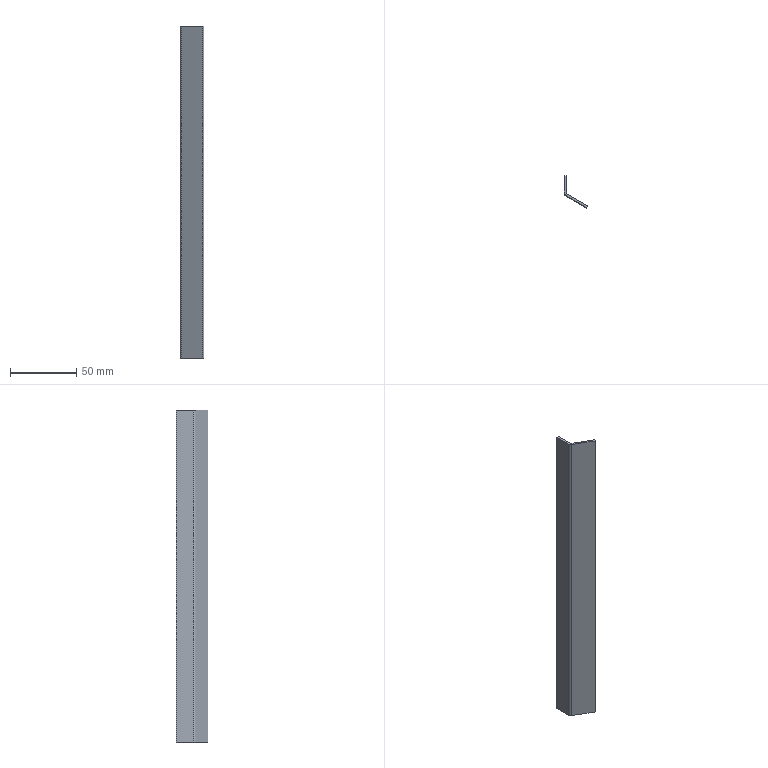Part | SolidWorks | features FlatPattern 1, SMBaseFlange 1, SheetMetal 1 | 1 solid | 14 faces | box 17.897 x 24.1 x 251.3 mm | volume 12439 mm3 | plane 12 | cylinder 2 | commonest cylinder face diameters 1 x1 4 x1
STEP:
#1=CARTESIAN_POINT('',(17.524,21.389,251.3));
#2=VERTEX_POINT('',#1);
#3=CARTESIAN_POINT('',(19.024,21.389,251.3));
#4=VERTEX_POINT('',#3);
#5=CARTESIAN_POINT('',(17.524,21.389,251.3));
#6=DIRECTION('',(1.,0.,0.));
#7=VECTOR('',#6,1000.);
#8=LINE('',#5,#7);
#9=EDGE_CURVE('',#2,#4,#8,.T.);
#10=ORIENTED_EDGE('',*,*,#9,.F.);
#11=CARTESIAN_POINT('',(18.524,19.657,251.3));
#12=VERTEX_POINT('',#11);
#13=CARTESIAN_POINT('',(19.524,21.389,251.3));
#14=DIRECTION('',(0.,0.,1.));
#15=DIRECTION('',(-1.,0.,0.));
#16=AXIS2_PLACEMENT_3D('',#13,#14,#15);
#17=CIRCLE('',#16,2.);
#18=EDGE_CURVE('',#2,#12,#17,.T.);
#19=ORIENTED_EDGE('',*,*,#18,.T.);
#20=CARTESIAN_POINT('',(19.274,20.956,251.3));
#21=VERTEX_POINT('',#20);
#22=CARTESIAN_POINT('',(19.274,20.956,251.3));
#23=DIRECTION('',(-0.5,-0.866,0.));
#24=VECTOR('',#23,1000.);
#25=LINE('',#22,#24);
#26=EDGE_CURVE('',#21,#12,#25,.T.);
#27=ORIENTED_EDGE('',*,*,#26,.F.);
#28=CARTESIAN_POINT('',(19.524,21.389,251.3));
#29=DIRECTION('',(0.,0.,1.));
#30=DIRECTION('',(1.,0.,0.));
#31=AXIS2_PLACEMENT_3D('',#28,#29,#30);
#32=CIRCLE('',#31,0.5);
#33=EDGE_CURVE('',#4,#21,#32,.T.);
#34=ORIENTED_EDGE('',*,*,#33,.F.);
#35=EDGE_LOOP('',(#10,#19,#27,#34));
#36=FACE_OUTER_BOUND('',#35,.T.);
#37=CARTESIAN_POINT('',(17.524,21.389,251.3));
#38=DIRECTION('',(0.,0.,1.));
#39=DIRECTION('',(1.,0.,0.));
#40=AXIS2_PLACEMENT_3D('',#37,#38,#39);
#41=PLANE('',#40);
#42=ADVANCED_FACE('',(#36),#41,.T.);
#43=CARTESIAN_POINT('',(17.524,34.435,251.3));
#44=VERTEX_POINT('',#43);
#45=CARTESIAN_POINT('',(17.524,34.435,251.3));
#46=DIRECTION('',(0.,-1.,0.));
#47=VECTOR('',#46,1000.);
#48=LINE('',#45,#47);
#49=EDGE_CURVE('',#44,#2,#48,.T.);
#50=ORIENTED_EDGE('',*,*,#49,.T.);
#51=ORIENTED_EDGE('',*,*,#9,.T.);
#52=CARTESIAN_POINT('',(19.024,34.435,251.3));
#53=VERTEX_POINT('',#52);
#54=CARTESIAN_POINT('',(19.024,34.435,251.3));
#55=DIRECTION('',(0.,-1.,0.));
#56=VECTOR('',#55,1000.);
#57=LINE('',#54,#56);
#58=EDGE_CURVE('',#53,#4,#57,.T.);
#59=ORIENTED_EDGE('',*,*,#58,.F.);
#60=CARTESIAN_POINT('',(17.524,34.435,251.3));
#61=DIRECTION('',(1.,0.,0.));
#62=VECTOR('',#61,1000.);
#63=LINE('',#60,#62);
#64=EDGE_CURVE('',#44,#53,#63,.T.);
#65=ORIENTED_EDGE('',*,*,#64,.F.);
#66=EDGE_LOOP('',(#50,#51,#59,#65));
#67=FACE_OUTER_BOUND('',#66,.T.);
#68=CARTESIAN_POINT('',(19.274,20.956,251.3));
#69=DIRECTION('',(0.,0.,1.));
#70=DIRECTION('',(1.,0.,0.));
#71=AXIS2_PLACEMENT_3D('',#68,#69,#70);
#72=PLANE('',#71);
#73=ADVANCED_FACE('',(#67),#72,.T.);
#74=CARTESIAN_POINT('',(18.524,19.657,0.));
#75=VERTEX_POINT('',#74);
#76=CARTESIAN_POINT('',(19.274,20.956,0.));
#77=VERTEX_POINT('',#76);
#78=CARTESIAN_POINT('',(18.524,19.657,0.));
#79=DIRECTION('',(0.5,0.866,0.));
#80=VECTOR('',#79,1000.);
#81=LINE('',#78,#80);
#82=EDGE_CURVE('',#75,#77,#81,.T.);
#83=ORIENTED_EDGE('',*,*,#82,.F.);
#84=CARTESIAN_POINT('',(17.524,21.389,0.));
#85=VERTEX_POINT('',#84);
#86=CARTESIAN_POINT('',(19.524,21.389,0.));
#87=DIRECTION('',(0.,0.,1.));
#88=DIRECTION('',(-1.,0.,0.));
#89=AXIS2_PLACEMENT_3D('',#86,#87,#88);
#90=CIRCLE('',#89,2.);
#91=EDGE_CURVE('',#85,#75,#90,.T.);
#92=ORIENTED_EDGE('',*,*,#91,.F.);
#93=CARTESIAN_POINT('',(19.024,21.389,0.));
#94=VERTEX_POINT('',#93);
#95=CARTESIAN_POINT('',(19.024,21.389,0.));
#96=DIRECTION('',(-1.,0.,0.));
#97=VECTOR('',#96,1000.);
#98=LINE('',#95,#97);
#99=EDGE_CURVE('',#94,#85,#98,.T.);
#100=ORIENTED_EDGE('',*,*,#99,.F.);
#101=CARTESIAN_POINT('',(19.524,21.389,0.));
#102=DIRECTION('',(0.,0.,1.));
#103=DIRECTION('',(1.,0.,0.));
#104=AXIS2_PLACEMENT_3D('',#101,#102,#103);
#105=CIRCLE('',#104,0.5);
#106=EDGE_CURVE('',#94,#77,#105,.T.);
#107=ORIENTED_EDGE('',*,*,#106,.T.);
#108=EDGE_LOOP('',(#83,#92,#100,#107));
#109=FACE_OUTER_BOUND('',#108,.T.);
#110=CARTESIAN_POINT('',(18.524,19.657,0.));
#111=DIRECTION('',(0.,0.,-1.));
#112=DIRECTION('',(-1.,0.,0.));
#113=AXIS2_PLACEMENT_3D('',#110,#111,#112);
#114=PLANE('',#113);
#115=ADVANCED_FACE('',(#109),#114,.T.);
#116=CARTESIAN_POINT('',(34.671,10.335,0.));
#117=VERTEX_POINT('',#116);
#118=CARTESIAN_POINT('',(17.524,20.235,0.));
#119=DIRECTION('',(0.866,-0.5,0.));
#120=VECTOR('',#119,1000.);
#121=LINE('',#118,#120);
#122=EDGE_CURVE('',#75,#117,#121,.T.);
#123=ORIENTED_EDGE('',*,*,#122,.F.);
#124=ORIENTED_EDGE('',*,*,#82,.T.);
#125=CARTESIAN_POINT('',(35.421,11.634,0.));
#126=VERTEX_POINT('',#125);
#127=CARTESIAN_POINT('',(18.274,21.534,0.));
#128=DIRECTION('',(0.866,-0.5,0.));
#129=VECTOR('',#128,1000.);
#130=LINE('',#127,#129);
#131=EDGE_CURVE('',#77,#126,#130,.T.);
#132=ORIENTED_EDGE('',*,*,#131,.T.);
#133=CARTESIAN_POINT('',(35.421,11.634,0.));
#134=DIRECTION('',(-0.5,-0.866,0.));
#135=VECTOR('',#134,1000.);
#136=LINE('',#133,#135);
#137=EDGE_CURVE('',#126,#117,#136,.T.);
#138=ORIENTED_EDGE('',*,*,#137,.T.);
#139=EDGE_LOOP('',(#123,#124,#132,#138));
#140=FACE_OUTER_BOUND('',#139,.T.);
#141=CARTESIAN_POINT('',(19.024,21.389,0.));
#142=DIRECTION('',(0.,0.,-1.));
#143=DIRECTION('',(-1.,0.,0.));
#144=AXIS2_PLACEMENT_3D('',#141,#142,#143);
#145=PLANE('',#144);
#146=ADVANCED_FACE('',(#140),#145,.T.);
#147=ORIENTED_EDGE('',*,*,#122,.T.);
#148=CARTESIAN_POINT('',(34.671,10.335,251.3));
#149=VERTEX_POINT('',#148);
#150=CARTESIAN_POINT('',(34.671,10.335,251.3));
#151=DIRECTION('',(0.,0.,-1.));
#152=VECTOR('',#151,1000.);
#153=LINE('',#150,#152);
#154=EDGE_CURVE('',#149,#117,#153,.T.);
#155=ORIENTED_EDGE('',*,*,#154,.F.);
#156=CARTESIAN_POINT('',(17.524,20.235,251.3));
#157=DIRECTION('',(0.866,-0.5,0.));
#158=VECTOR('',#157,1000.);
#159=LINE('',#156,#158);
#160=EDGE_CURVE('',#12,#149,#159,.T.);
#161=ORIENTED_EDGE('',*,*,#160,.F.);
#162=CARTESIAN_POINT('',(18.524,19.657,251.3));
#163=DIRECTION('',(0.,0.,-1.));
#164=VECTOR('',#163,1000.);
#165=LINE('',#162,#164);
#166=EDGE_CURVE('',#12,#75,#165,.T.);
#167=ORIENTED_EDGE('',*,*,#166,.T.);
#168=EDGE_LOOP('',(#147,#155,#161,#167));
#169=FACE_OUTER_BOUND('',#168,.T.);
#170=CARTESIAN_POINT('',(17.524,20.235,251.3));
#171=DIRECTION('',(0.5,0.866,0.));
#172=DIRECTION('',(-0.866,0.5,0.));
#173=AXIS2_PLACEMENT_3D('',#170,#171,#172);
#174=PLANE('',#173);
#175=ADVANCED_FACE('',(#169),#174,.F.);
#176=ORIENTED_EDGE('',*,*,#137,.F.);
#177=CARTESIAN_POINT('',(35.421,11.634,251.3));
#178=VERTEX_POINT('',#177);
#179=CARTESIAN_POINT('',(35.421,11.634,251.3));
#180=DIRECTION('',(0.,0.,-1.));
#181=VECTOR('',#180,1000.);
#182=LINE('',#179,#181);
#183=EDGE_CURVE('',#178,#126,#182,.T.);
#184=ORIENTED_EDGE('',*,*,#183,.F.);
#185=CARTESIAN_POINT('',(35.421,11.634,251.3));
#186=DIRECTION('',(-0.5,-0.866,0.));
#187=VECTOR('',#186,1000.);
#188=LINE('',#185,#187);
#189=EDGE_CURVE('',#178,#149,#188,.T.);
#190=ORIENTED_EDGE('',*,*,#189,.T.);
#191=ORIENTED_EDGE('',*,*,#154,.T.);
#192=EDGE_LOOP('',(#176,#184,#190,#191));
#193=FACE_OUTER_BOUND('',#192,.T.);
#194=CARTESIAN_POINT('',(35.421,11.634,251.3));
#195=DIRECTION('',(0.866,-0.5,0.));
#196=DIRECTION('',(0.5,0.866,0.));
#197=AXIS2_PLACEMENT_3D('',#194,#195,#196);
#198=PLANE('',#197);
#199=ADVANCED_FACE('',(#193),#198,.T.);
#200=ORIENTED_EDGE('',*,*,#131,.F.);
#201=CARTESIAN_POINT('',(19.274,20.956,251.3));
#202=DIRECTION('',(0.,0.,-1.));
#203=VECTOR('',#202,1000.);
#204=LINE('',#201,#203);
#205=EDGE_CURVE('',#21,#77,#204,.T.);
#206=ORIENTED_EDGE('',*,*,#205,.F.);
#207=CARTESIAN_POINT('',(18.274,21.534,251.3));
#208=DIRECTION('',(0.866,-0.5,0.));
#209=VECTOR('',#208,1000.);
#210=LINE('',#207,#209);
#211=EDGE_CURVE('',#21,#178,#210,.T.);
#212=ORIENTED_EDGE('',*,*,#211,.T.);
#213=ORIENTED_EDGE('',*,*,#183,.T.);
#214=EDGE_LOOP('',(#200,#206,#212,#213));
#215=FACE_OUTER_BOUND('',#214,.T.);
#216=CARTESIAN_POINT('',(18.274,21.534,251.3));
#217=DIRECTION('',(0.5,0.866,0.));
#218=DIRECTION('',(-0.866,0.5,0.));
#219=AXIS2_PLACEMENT_3D('',#216,#217,#218);
#220=PLANE('',#219);
#221=ADVANCED_FACE('',(#215),#220,.T.);
#222=ORIENTED_EDGE('',*,*,#106,.F.);
#223=CARTESIAN_POINT('',(19.024,21.389,251.3));
#224=DIRECTION('',(0.,0.,-1.));
#225=VECTOR('',#224,1000.);
#226=LINE('',#223,#225);
#227=EDGE_CURVE('',#4,#94,#226,.T.);
#228=ORIENTED_EDGE('',*,*,#227,.F.);
#229=ORIENTED_EDGE('',*,*,#33,.T.);
#230=ORIENTED_EDGE('',*,*,#205,.T.);
#231=EDGE_LOOP('',(#222,#228,#229,#230));
#232=FACE_OUTER_BOUND('',#231,.T.);
#233=CARTESIAN_POINT('',(19.524,21.389,251.3));
#234=DIRECTION('',(0.,0.,-1.));
#235=DIRECTION('',(-1.,0.,0.));
#236=AXIS2_PLACEMENT_3D('',#233,#234,#235);
#237=CYLINDRICAL_SURFACE('',#236,0.5);
#238=ADVANCED_FACE('',(#232),#237,.F.);
#239=CARTESIAN_POINT('',(19.024,34.435,0.));
#240=VERTEX_POINT('',#239);
#241=CARTESIAN_POINT('',(19.024,34.435,0.));
#242=DIRECTION('',(0.,-1.,0.));
#243=VECTOR('',#242,1000.);
#244=LINE('',#241,#243);
#245=EDGE_CURVE('',#240,#94,#244,.T.);
#246=ORIENTED_EDGE('',*,*,#245,.F.);
#247=CARTESIAN_POINT('',(19.024,34.435,251.3));
#248=DIRECTION('',(0.,0.,-1.));
#249=VECTOR('',#248,1000.);
#250=LINE('',#247,#249);
#251=EDGE_CURVE('',#53,#240,#250,.T.);
#252=ORIENTED_EDGE('',*,*,#251,.F.);
#253=ORIENTED_EDGE('',*,*,#58,.T.);
#254=ORIENTED_EDGE('',*,*,#227,.T.);
#255=EDGE_LOOP('',(#246,#252,#253,#254));
#256=FACE_OUTER_BOUND('',#255,.T.);
#257=CARTESIAN_POINT('',(19.024,34.435,251.3));
#258=DIRECTION('',(1.,0.,0.));
#259=DIRECTION('',(0.,0.,-1.));
#260=AXIS2_PLACEMENT_3D('',#257,#258,#259);
#261=PLANE('',#260);
#262=ADVANCED_FACE('',(#256),#261,.T.);
#263=CARTESIAN_POINT('',(17.524,34.435,0.));
#264=VERTEX_POINT('',#263);
#265=CARTESIAN_POINT('',(17.524,34.435,0.));
#266=DIRECTION('',(1.,0.,0.));
#267=VECTOR('',#266,1000.);
#268=LINE('',#265,#267);
#269=EDGE_CURVE('',#264,#240,#268,.T.);
#270=ORIENTED_EDGE('',*,*,#269,.F.);
#271=CARTESIAN_POINT('',(17.524,34.435,251.3));
#272=DIRECTION('',(0.,0.,-1.));
#273=VECTOR('',#272,1000.);
#274=LINE('',#271,#273);
#275=EDGE_CURVE('',#44,#264,#274,.T.);
#276=ORIENTED_EDGE('',*,*,#275,.F.);
#277=ORIENTED_EDGE('',*,*,#64,.T.);
#278=ORIENTED_EDGE('',*,*,#251,.T.);
#279=EDGE_LOOP('',(#270,#276,#277,#278));
#280=FACE_OUTER_BOUND('',#279,.T.);
#281=CARTESIAN_POINT('',(17.524,34.435,251.3));
#282=DIRECTION('',(0.,1.,0.));
#283=DIRECTION('',(0.,0.,1.));
#284=AXIS2_PLACEMENT_3D('',#281,#282,#283);
#285=PLANE('',#284);
#286=ADVANCED_FACE('',(#280),#285,.T.);
#287=CARTESIAN_POINT('',(17.524,34.435,0.));
#288=DIRECTION('',(0.,-1.,0.));
#289=VECTOR('',#288,1000.);
#290=LINE('',#287,#289);
#291=EDGE_CURVE('',#264,#85,#290,.T.);
#292=ORIENTED_EDGE('',*,*,#291,.T.);
#293=CARTESIAN_POINT('',(17.524,21.389,251.3));
#294=DIRECTION('',(0.,0.,-1.));
#295=VECTOR('',#294,1000.);
#296=LINE('',#293,#295);
#297=EDGE_CURVE('',#2,#85,#296,.T.);
#298=ORIENTED_EDGE('',*,*,#297,.F.);
#299=ORIENTED_EDGE('',*,*,#49,.F.);
#300=ORIENTED_EDGE('',*,*,#275,.T.);
#301=EDGE_LOOP('',(#292,#298,#299,#300));
#302=FACE_OUTER_BOUND('',#301,.T.);
#303=CARTESIAN_POINT('',(17.524,34.435,251.3));
#304=DIRECTION('',(1.,0.,0.));
#305=DIRECTION('',(0.,0.,-1.));
#306=AXIS2_PLACEMENT_3D('',#303,#304,#305);
#307=PLANE('',#306);
#308=ADVANCED_FACE('',(#302),#307,.F.);
#309=ORIENTED_EDGE('',*,*,#91,.T.);
#310=ORIENTED_EDGE('',*,*,#166,.F.);
#311=ORIENTED_EDGE('',*,*,#18,.F.);
#312=ORIENTED_EDGE('',*,*,#297,.T.);
#313=EDGE_LOOP('',(#309,#310,#311,#312));
#314=FACE_OUTER_BOUND('',#313,.T.);
#315=CARTESIAN_POINT('',(19.524,21.389,251.3));
#316=DIRECTION('',(0.,0.,-1.));
#317=DIRECTION('',(-1.,0.,0.));
#318=AXIS2_PLACEMENT_3D('',#315,#316,#317);
#319=CYLINDRICAL_SURFACE('',#318,2.);
#320=ADVANCED_FACE('',(#314),#319,.T.);
#321=ORIENTED_EDGE('',*,*,#160,.T.);
#322=ORIENTED_EDGE('',*,*,#189,.F.);
#323=ORIENTED_EDGE('',*,*,#211,.F.);
#324=ORIENTED_EDGE('',*,*,#26,.T.);
#325=EDGE_LOOP('',(#321,#322,#323,#324));
#326=FACE_OUTER_BOUND('',#325,.T.);
#327=CARTESIAN_POINT('',(19.524,21.389,251.3));
#328=DIRECTION('',(0.,0.,1.));
#329=DIRECTION('',(1.,0.,0.));
#330=AXIS2_PLACEMENT_3D('',#327,#328,#329);
#331=PLANE('',#330);
#332=ADVANCED_FACE('',(#326),#331,.T.);
#333=ORIENTED_EDGE('',*,*,#245,.T.);
#334=ORIENTED_EDGE('',*,*,#99,.T.);
#335=ORIENTED_EDGE('',*,*,#291,.F.);
#336=ORIENTED_EDGE('',*,*,#269,.T.);
#337=EDGE_LOOP('',(#333,#334,#335,#336));
#338=FACE_OUTER_BOUND('',#337,.T.);
#339=CARTESIAN_POINT('',(19.524,21.389,0.));
#340=DIRECTION('',(0.,0.,1.));
#341=DIRECTION('',(1.,0.,0.));
#342=AXIS2_PLACEMENT_3D('',#339,#340,#341);
#343=PLANE('',#342);
#344=ADVANCED_FACE('',(#338),#343,.F.);
#345=CLOSED_SHELL('',(#42,#73,#115,#146,#175,#199,#221,#238,#262,#286,#308,#320,#332,#344));
#346=MANIFOLD_SOLID_BREP('',#345);
#347=CARTESIAN_POINT('',(0.,0.,0.));
#348=DIRECTION('',(0.,0.,1.));
#349=DIRECTION('',(1.,0.,0.));
#350=AXIS2_PLACEMENT_3D('',#347,#348,#349);
#351=(LENGTH_UNIT()NAMED_UNIT(*)SI_UNIT(.MILLI.,.METRE.));
#352=UNCERTAINTY_MEASURE_WITH_UNIT(LENGTH_MEASURE(0.00001),#351,'','');
#353=(NAMED_UNIT(*)PLANE_ANGLE_UNIT()SI_UNIT($,.RADIAN.));
#354=(NAMED_UNIT(*)SI_UNIT($,.STERADIAN.)SOLID_ANGLE_UNIT());
#355=(GEOMETRIC_REPRESENTATION_CONTEXT(3)GLOBAL_UNCERTAINTY_ASSIGNED_CONTEXT((#352))GLOBAL_UNIT_ASSIGNED_CONTEXT((#351,#353,#354))REPRESENTATION_CONTEXT('',''));
#356=ADVANCED_BREP_SHAPE_REPRESENTATION('',(#346,#350),#355);